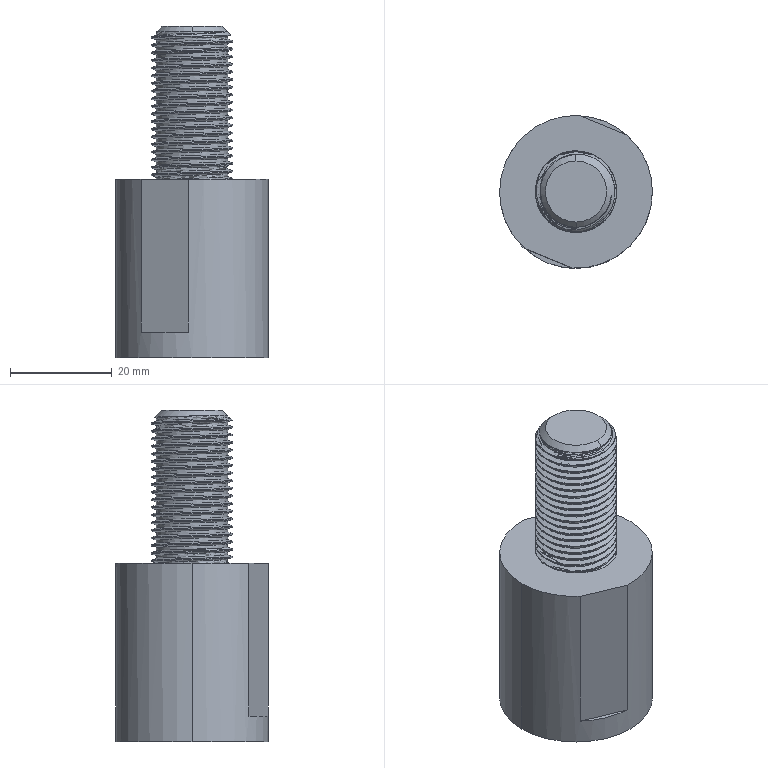Part | SolidWorks | features BaseBody 1 | 1 solid | 58 faces | box 30 x 30 x 65 mm | volume 25106 mm3 | cylinder 43 | plane 7 | cone 5 | spline 3 | commonest cylinder face diameters 16 x39 14.5 x2 30 x2